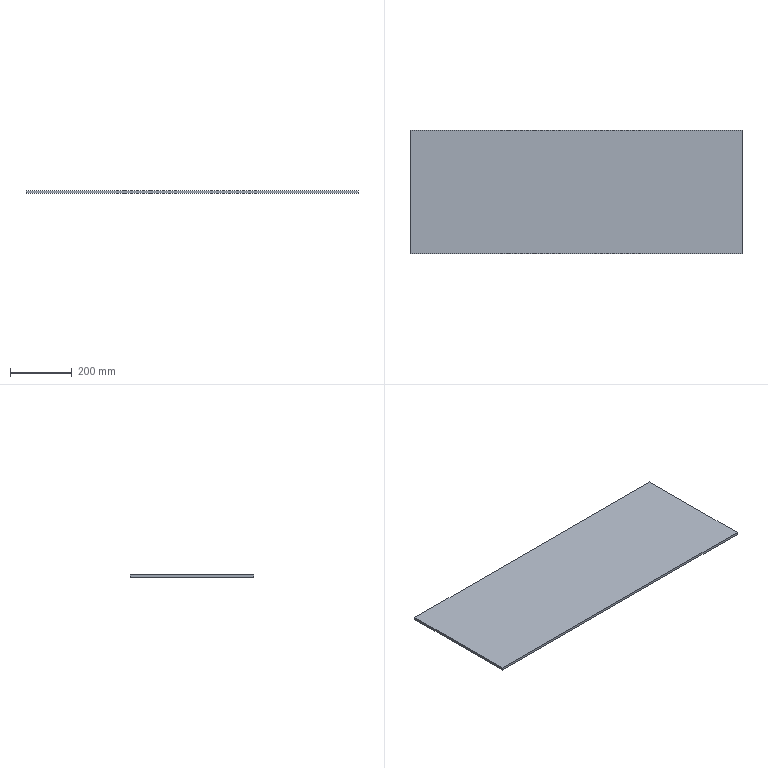Part | STEP file | Rear baffle 1079X402X8_Default<As machined> | 1 solid | 6 faces | box 1079 x 402 x 8 mm | volume 3470064 mm3 | plane 6
STEP:
#1=CARTESIAN_POINT('',(0.,0.,0.));
#2=DIRECTION('',(0.,0.,1.));
#3=DIRECTION('',(1.,0.,0.));
#4=AXIS2_PLACEMENT_3D('',#1,#2,#3);
#5=CARTESIAN_POINT('',(539.5,-201.,0.));
#6=VERTEX_POINT('',#5);
#7=CARTESIAN_POINT('',(539.5,201.,0.));
#8=VERTEX_POINT('',#7);
#9=CARTESIAN_POINT('',(539.5,201.,0.));
#10=DIRECTION('',(0.,1.,0.));
#11=VECTOR('',#10,1.);
#12=LINE('',#9,#11);
#13=CARTESIAN_POINT('',(539.5,201.,8.));
#14=DIRECTION('',(-1.,0.,0.));
#15=DIRECTION('',(0.,0.,1.));
#16=AXIS2_PLACEMENT_3D('',#13,#14,#15);
#17=PLANE('',#16);
#18=CARTESIAN_POINT('',(-8.,0.));
#19=DIRECTION('',(0.,1.));
#20=VECTOR('',#19,1.);
#21=LINE('',#18,#20);
#22=(GEOMETRIC_REPRESENTATION_CONTEXT(2)PARAMETRIC_REPRESENTATION_CONTEXT()REPRESENTATION_CONTEXT('',''));
#23=DEFINITIONAL_REPRESENTATION('',(#21),#22);
#24=PCURVE('',#17,#23);
#25=CARTESIAN_POINT('',(0.,0.,0.));
#26=DIRECTION('',(0.,0.,1.));
#27=DIRECTION('',(1.,0.,0.));
#28=AXIS2_PLACEMENT_3D('',#25,#26,#27);
#29=PLANE('',#28);
#30=CARTESIAN_POINT('',(539.5,201.));
#31=DIRECTION('',(0.,1.));
#32=VECTOR('',#31,1.);
#33=LINE('',#30,#32);
#34=(GEOMETRIC_REPRESENTATION_CONTEXT(2)PARAMETRIC_REPRESENTATION_CONTEXT()REPRESENTATION_CONTEXT('',''));
#35=DEFINITIONAL_REPRESENTATION('',(#33),#34);
#36=PCURVE('',#29,#35);
#37=SURFACE_CURVE('',#12,(#24,#36),.PCURVE_S1.);
#38=EDGE_CURVE('',#6,#8,#37,.T.);
#39=ORIENTED_EDGE('',*,*,#38,.T.);
#40=CARTESIAN_POINT('',(539.5,201.,8.));
#41=VERTEX_POINT('',#40);
#42=CARTESIAN_POINT('',(539.5,201.,8.));
#43=DIRECTION('',(0.,0.,-1.));
#44=VECTOR('',#43,1.);
#45=LINE('',#42,#44);
#46=CARTESIAN_POINT('',(0.,0.));
#47=DIRECTION('',(-1.,0.));
#48=VECTOR('',#47,1.);
#49=LINE('',#46,#48);
#50=(GEOMETRIC_REPRESENTATION_CONTEXT(2)PARAMETRIC_REPRESENTATION_CONTEXT()REPRESENTATION_CONTEXT('',''));
#51=DEFINITIONAL_REPRESENTATION('',(#49),#50);
#52=PCURVE('',#17,#51);
#53=CARTESIAN_POINT('',(-539.5,201.,8.));
#54=DIRECTION('',(0.,-1.,0.));
#55=DIRECTION('',(0.,0.,-1.));
#56=AXIS2_PLACEMENT_3D('',#53,#54,#55);
#57=PLANE('',#56);
#58=CARTESIAN_POINT('',(0.,1079.));
#59=DIRECTION('',(1.,0.));
#60=VECTOR('',#59,1.);
#61=LINE('',#58,#60);
#62=(GEOMETRIC_REPRESENTATION_CONTEXT(2)PARAMETRIC_REPRESENTATION_CONTEXT()REPRESENTATION_CONTEXT('',''));
#63=DEFINITIONAL_REPRESENTATION('',(#61),#62);
#64=PCURVE('',#57,#63);
#65=SURFACE_CURVE('',#45,(#52,#64),.PCURVE_S1.);
#66=EDGE_CURVE('',#41,#8,#65,.T.);
#67=ORIENTED_EDGE('',*,*,#66,.F.);
#68=CARTESIAN_POINT('',(539.5,-201.,8.));
#69=VERTEX_POINT('',#68);
#70=CARTESIAN_POINT('',(539.5,201.,8.));
#71=DIRECTION('',(0.,1.,0.));
#72=VECTOR('',#71,1.);
#73=LINE('',#70,#72);
#74=CARTESIAN_POINT('',(0.,0.));
#75=DIRECTION('',(0.,1.));
#76=VECTOR('',#75,1.);
#77=LINE('',#74,#76);
#78=(GEOMETRIC_REPRESENTATION_CONTEXT(2)PARAMETRIC_REPRESENTATION_CONTEXT()REPRESENTATION_CONTEXT('',''));
#79=DEFINITIONAL_REPRESENTATION('',(#77),#78);
#80=PCURVE('',#17,#79);
#81=CARTESIAN_POINT('',(0.,0.,8.));
#82=DIRECTION('',(0.,0.,1.));
#83=DIRECTION('',(1.,0.,0.));
#84=AXIS2_PLACEMENT_3D('',#81,#82,#83);
#85=PLANE('',#84);
#86=CARTESIAN_POINT('',(539.5,201.));
#87=DIRECTION('',(0.,1.));
#88=VECTOR('',#87,1.);
#89=LINE('',#86,#88);
#90=(GEOMETRIC_REPRESENTATION_CONTEXT(2)PARAMETRIC_REPRESENTATION_CONTEXT()REPRESENTATION_CONTEXT('',''));
#91=DEFINITIONAL_REPRESENTATION('',(#89),#90);
#92=PCURVE('',#85,#91);
#93=SURFACE_CURVE('',#73,(#80,#92),.PCURVE_S1.);
#94=EDGE_CURVE('',#69,#41,#93,.T.);
#95=ORIENTED_EDGE('',*,*,#94,.F.);
#96=CARTESIAN_POINT('',(539.5,-201.,8.));
#97=DIRECTION('',(0.,0.,-1.));
#98=VECTOR('',#97,1.);
#99=LINE('',#96,#98);
#100=CARTESIAN_POINT('',(0.,-402.));
#101=DIRECTION('',(-1.,0.));
#102=VECTOR('',#101,1.);
#103=LINE('',#100,#102);
#104=(GEOMETRIC_REPRESENTATION_CONTEXT(2)PARAMETRIC_REPRESENTATION_CONTEXT()REPRESENTATION_CONTEXT('',''));
#105=DEFINITIONAL_REPRESENTATION('',(#103),#104);
#106=PCURVE('',#17,#105);
#107=CARTESIAN_POINT('',(-539.5,-201.,8.));
#108=DIRECTION('',(0.,1.,0.));
#109=DIRECTION('',(0.,0.,1.));
#110=AXIS2_PLACEMENT_3D('',#107,#108,#109);
#111=PLANE('',#110);
#112=CARTESIAN_POINT('',(0.,1079.));
#113=DIRECTION('',(-1.,0.));
#114=VECTOR('',#113,1.);
#115=LINE('',#112,#114);
#116=(GEOMETRIC_REPRESENTATION_CONTEXT(2)PARAMETRIC_REPRESENTATION_CONTEXT()REPRESENTATION_CONTEXT('',''));
#117=DEFINITIONAL_REPRESENTATION('',(#115),#116);
#118=PCURVE('',#111,#117);
#119=SURFACE_CURVE('',#99,(#106,#118),.PCURVE_S1.);
#120=EDGE_CURVE('',#69,#6,#119,.T.);
#121=ORIENTED_EDGE('',*,*,#120,.T.);
#122=EDGE_LOOP('',(#39,#67,#95,#121));
#123=FACE_BOUND('',#122,.T.);
#124=ADVANCED_FACE('',(#123),#17,.F.);
#125=CARTESIAN_POINT('',(-539.5,201.,0.));
#126=VERTEX_POINT('',#125);
#127=CARTESIAN_POINT('',(-539.5,201.,0.));
#128=DIRECTION('',(-1.,0.,0.));
#129=VECTOR('',#128,1.);
#130=LINE('',#127,#129);
#131=CARTESIAN_POINT('',(8.,0.));
#132=DIRECTION('',(0.,-1.));
#133=VECTOR('',#132,1.);
#134=LINE('',#131,#133);
#135=(GEOMETRIC_REPRESENTATION_CONTEXT(2)PARAMETRIC_REPRESENTATION_CONTEXT()REPRESENTATION_CONTEXT('',''));
#136=DEFINITIONAL_REPRESENTATION('',(#134),#135);
#137=PCURVE('',#57,#136);
#138=CARTESIAN_POINT('',(-539.5,201.));
#139=DIRECTION('',(-1.,0.));
#140=VECTOR('',#139,1.);
#141=LINE('',#138,#140);
#142=(GEOMETRIC_REPRESENTATION_CONTEXT(2)PARAMETRIC_REPRESENTATION_CONTEXT()REPRESENTATION_CONTEXT('',''));
#143=DEFINITIONAL_REPRESENTATION('',(#141),#142);
#144=PCURVE('',#29,#143);
#145=SURFACE_CURVE('',#130,(#137,#144),.PCURVE_S1.);
#146=EDGE_CURVE('',#8,#126,#145,.T.);
#147=ORIENTED_EDGE('',*,*,#146,.T.);
#148=CARTESIAN_POINT('',(-539.5,201.,8.));
#149=VERTEX_POINT('',#148);
#150=CARTESIAN_POINT('',(-539.5,201.,8.));
#151=DIRECTION('',(0.,0.,-1.));
#152=VECTOR('',#151,1.);
#153=LINE('',#150,#152);
#154=CARTESIAN_POINT('',(0.,0.));
#155=DIRECTION('',(1.,0.));
#156=VECTOR('',#155,1.);
#157=LINE('',#154,#156);
#158=(GEOMETRIC_REPRESENTATION_CONTEXT(2)PARAMETRIC_REPRESENTATION_CONTEXT()REPRESENTATION_CONTEXT('',''));
#159=DEFINITIONAL_REPRESENTATION('',(#157),#158);
#160=PCURVE('',#57,#159);
#161=CARTESIAN_POINT('',(-539.5,201.,8.));
#162=DIRECTION('',(1.,0.,0.));
#163=DIRECTION('',(0.,1.,0.));
#164=AXIS2_PLACEMENT_3D('',#161,#162,#163);
#165=PLANE('',#164);
#166=CARTESIAN_POINT('',(0.,0.));
#167=DIRECTION('',(0.,-1.));
#168=VECTOR('',#167,1.);
#169=LINE('',#166,#168);
#170=(GEOMETRIC_REPRESENTATION_CONTEXT(2)PARAMETRIC_REPRESENTATION_CONTEXT()REPRESENTATION_CONTEXT('',''));
#171=DEFINITIONAL_REPRESENTATION('',(#169),#170);
#172=PCURVE('',#165,#171);
#173=SURFACE_CURVE('',#153,(#160,#172),.PCURVE_S1.);
#174=EDGE_CURVE('',#149,#126,#173,.T.);
#175=ORIENTED_EDGE('',*,*,#174,.F.);
#176=CARTESIAN_POINT('',(-539.5,201.,8.));
#177=DIRECTION('',(-1.,0.,0.));
#178=VECTOR('',#177,1.);
#179=LINE('',#176,#178);
#180=CARTESIAN_POINT('',(0.,0.));
#181=DIRECTION('',(0.,-1.));
#182=VECTOR('',#181,1.);
#183=LINE('',#180,#182);
#184=(GEOMETRIC_REPRESENTATION_CONTEXT(2)PARAMETRIC_REPRESENTATION_CONTEXT()REPRESENTATION_CONTEXT('',''));
#185=DEFINITIONAL_REPRESENTATION('',(#183),#184);
#186=PCURVE('',#57,#185);
#187=CARTESIAN_POINT('',(-539.5,201.));
#188=DIRECTION('',(-1.,0.));
#189=VECTOR('',#188,1.);
#190=LINE('',#187,#189);
#191=(GEOMETRIC_REPRESENTATION_CONTEXT(2)PARAMETRIC_REPRESENTATION_CONTEXT()REPRESENTATION_CONTEXT('',''));
#192=DEFINITIONAL_REPRESENTATION('',(#190),#191);
#193=PCURVE('',#85,#192);
#194=SURFACE_CURVE('',#179,(#186,#193),.PCURVE_S1.);
#195=EDGE_CURVE('',#41,#149,#194,.T.);
#196=ORIENTED_EDGE('',*,*,#195,.F.);
#197=ORIENTED_EDGE('',*,*,#66,.T.);
#198=EDGE_LOOP('',(#147,#175,#196,#197));
#199=FACE_BOUND('',#198,.T.);
#200=ADVANCED_FACE('',(#199),#57,.F.);
#201=CARTESIAN_POINT('',(-539.5,-201.,0.));
#202=VERTEX_POINT('',#201);
#203=CARTESIAN_POINT('',(-539.5,201.,0.));
#204=DIRECTION('',(0.,-1.,0.));
#205=VECTOR('',#204,1.);
#206=LINE('',#203,#205);
#207=CARTESIAN_POINT('',(0.,-8.));
#208=DIRECTION('',(-1.,0.));
#209=VECTOR('',#208,1.);
#210=LINE('',#207,#209);
#211=(GEOMETRIC_REPRESENTATION_CONTEXT(2)PARAMETRIC_REPRESENTATION_CONTEXT()REPRESENTATION_CONTEXT('',''));
#212=DEFINITIONAL_REPRESENTATION('',(#210),#211);
#213=PCURVE('',#165,#212);
#214=CARTESIAN_POINT('',(-539.5,201.));
#215=DIRECTION('',(0.,-1.));
#216=VECTOR('',#215,1.);
#217=LINE('',#214,#216);
#218=(GEOMETRIC_REPRESENTATION_CONTEXT(2)PARAMETRIC_REPRESENTATION_CONTEXT()REPRESENTATION_CONTEXT('',''));
#219=DEFINITIONAL_REPRESENTATION('',(#217),#218);
#220=PCURVE('',#29,#219);
#221=SURFACE_CURVE('',#206,(#213,#220),.PCURVE_S1.);
#222=EDGE_CURVE('',#126,#202,#221,.T.);
#223=ORIENTED_EDGE('',*,*,#222,.T.);
#224=CARTESIAN_POINT('',(-539.5,-201.,8.));
#225=VERTEX_POINT('',#224);
#226=CARTESIAN_POINT('',(-539.5,-201.,8.));
#227=DIRECTION('',(0.,0.,-1.));
#228=VECTOR('',#227,1.);
#229=LINE('',#226,#228);
#230=CARTESIAN_POINT('',(-402.,0.));
#231=DIRECTION('',(0.,-1.));
#232=VECTOR('',#231,1.);
#233=LINE('',#230,#232);
#234=(GEOMETRIC_REPRESENTATION_CONTEXT(2)PARAMETRIC_REPRESENTATION_CONTEXT()REPRESENTATION_CONTEXT('',''));
#235=DEFINITIONAL_REPRESENTATION('',(#233),#234);
#236=PCURVE('',#165,#235);
#237=CARTESIAN_POINT('',(0.,0.));
#238=DIRECTION('',(-1.,0.));
#239=VECTOR('',#238,1.);
#240=LINE('',#237,#239);
#241=(GEOMETRIC_REPRESENTATION_CONTEXT(2)PARAMETRIC_REPRESENTATION_CONTEXT()REPRESENTATION_CONTEXT('',''));
#242=DEFINITIONAL_REPRESENTATION('',(#240),#241);
#243=PCURVE('',#111,#242);
#244=SURFACE_CURVE('',#229,(#236,#243),.PCURVE_S1.);
#245=EDGE_CURVE('',#225,#202,#244,.T.);
#246=ORIENTED_EDGE('',*,*,#245,.F.);
#247=CARTESIAN_POINT('',(-539.5,201.,8.));
#248=DIRECTION('',(0.,-1.,0.));
#249=VECTOR('',#248,1.);
#250=LINE('',#247,#249);
#251=CARTESIAN_POINT('',(0.,0.));
#252=DIRECTION('',(-1.,0.));
#253=VECTOR('',#252,1.);
#254=LINE('',#251,#253);
#255=(GEOMETRIC_REPRESENTATION_CONTEXT(2)PARAMETRIC_REPRESENTATION_CONTEXT()REPRESENTATION_CONTEXT('',''));
#256=DEFINITIONAL_REPRESENTATION('',(#254),#255);
#257=PCURVE('',#165,#256);
#258=CARTESIAN_POINT('',(-539.5,201.));
#259=DIRECTION('',(0.,-1.));
#260=VECTOR('',#259,1.);
#261=LINE('',#258,#260);
#262=(GEOMETRIC_REPRESENTATION_CONTEXT(2)PARAMETRIC_REPRESENTATION_CONTEXT()REPRESENTATION_CONTEXT('',''));
#263=DEFINITIONAL_REPRESENTATION('',(#261),#262);
#264=PCURVE('',#85,#263);
#265=SURFACE_CURVE('',#250,(#257,#264),.PCURVE_S1.);
#266=EDGE_CURVE('',#149,#225,#265,.T.);
#267=ORIENTED_EDGE('',*,*,#266,.F.);
#268=ORIENTED_EDGE('',*,*,#174,.T.);
#269=EDGE_LOOP('',(#223,#246,#267,#268));
#270=FACE_BOUND('',#269,.T.);
#271=ADVANCED_FACE('',(#270),#165,.F.);
#272=CARTESIAN_POINT('',(-539.5,-201.,0.));
#273=DIRECTION('',(1.,0.,0.));
#274=VECTOR('',#273,1.);
#275=LINE('',#272,#274);
#276=CARTESIAN_POINT('',(-8.,0.));
#277=DIRECTION('',(0.,1.));
#278=VECTOR('',#277,1.);
#279=LINE('',#276,#278);
#280=(GEOMETRIC_REPRESENTATION_CONTEXT(2)PARAMETRIC_REPRESENTATION_CONTEXT()REPRESENTATION_CONTEXT('',''));
#281=DEFINITIONAL_REPRESENTATION('',(#279),#280);
#282=PCURVE('',#111,#281);
#283=CARTESIAN_POINT('',(-539.5,-201.));
#284=DIRECTION('',(1.,0.));
#285=VECTOR('',#284,1.);
#286=LINE('',#283,#285);
#287=(GEOMETRIC_REPRESENTATION_CONTEXT(2)PARAMETRIC_REPRESENTATION_CONTEXT()REPRESENTATION_CONTEXT('',''));
#288=DEFINITIONAL_REPRESENTATION('',(#286),#287);
#289=PCURVE('',#29,#288);
#290=SURFACE_CURVE('',#275,(#282,#289),.PCURVE_S1.);
#291=EDGE_CURVE('',#202,#6,#290,.T.);
#292=ORIENTED_EDGE('',*,*,#291,.T.);
#293=ORIENTED_EDGE('',*,*,#120,.F.);
#294=CARTESIAN_POINT('',(-539.5,-201.,8.));
#295=DIRECTION('',(1.,0.,0.));
#296=VECTOR('',#295,1.);
#297=LINE('',#294,#296);
#298=CARTESIAN_POINT('',(0.,0.));
#299=DIRECTION('',(0.,1.));
#300=VECTOR('',#299,1.);
#301=LINE('',#298,#300);
#302=(GEOMETRIC_REPRESENTATION_CONTEXT(2)PARAMETRIC_REPRESENTATION_CONTEXT()REPRESENTATION_CONTEXT('',''));
#303=DEFINITIONAL_REPRESENTATION('',(#301),#302);
#304=PCURVE('',#111,#303);
#305=CARTESIAN_POINT('',(-539.5,-201.));
#306=DIRECTION('',(1.,0.));
#307=VECTOR('',#306,1.);
#308=LINE('',#305,#307);
#309=(GEOMETRIC_REPRESENTATION_CONTEXT(2)PARAMETRIC_REPRESENTATION_CONTEXT()REPRESENTATION_CONTEXT('',''));
#310=DEFINITIONAL_REPRESENTATION('',(#308),#309);
#311=PCURVE('',#85,#310);
#312=SURFACE_CURVE('',#297,(#304,#311),.PCURVE_S1.);
#313=EDGE_CURVE('',#225,#69,#312,.T.);
#314=ORIENTED_EDGE('',*,*,#313,.F.);
#315=ORIENTED_EDGE('',*,*,#245,.T.);
#316=EDGE_LOOP('',(#292,#293,#314,#315));
#317=FACE_BOUND('',#316,.T.);
#318=ADVANCED_FACE('',(#317),#111,.F.);
#319=ORIENTED_EDGE('',*,*,#94,.T.);
#320=ORIENTED_EDGE('',*,*,#195,.T.);
#321=ORIENTED_EDGE('',*,*,#266,.T.);
#322=ORIENTED_EDGE('',*,*,#313,.T.);
#323=EDGE_LOOP('',(#319,#320,#321,#322));
#324=FACE_BOUND('',#323,.T.);
#325=ADVANCED_FACE('',(#324),#85,.T.);
#326=ORIENTED_EDGE('',*,*,#38,.F.);
#327=ORIENTED_EDGE('',*,*,#291,.F.);
#328=ORIENTED_EDGE('',*,*,#222,.F.);
#329=ORIENTED_EDGE('',*,*,#146,.F.);
#330=EDGE_LOOP('',(#326,#327,#328,#329));
#331=FACE_BOUND('',#330,.T.);
#332=ADVANCED_FACE('',(#331),#29,.F.);
#333=CLOSED_SHELL('',(#124,#200,#271,#318,#325,#332));
#334=MANIFOLD_SOLID_BREP('',#333);
#335=(LENGTH_UNIT()NAMED_UNIT(*)SI_UNIT(.MILLI.,.METRE.));
#336=UNCERTAINTY_MEASURE_WITH_UNIT(LENGTH_MEASURE(0.0000001),#335,'','');
#337=(NAMED_UNIT(*)PLANE_ANGLE_UNIT()SI_UNIT($,.RADIAN.));
#338=(NAMED_UNIT(*)SI_UNIT($,.STERADIAN.)SOLID_ANGLE_UNIT());
#339=(GEOMETRIC_REPRESENTATION_CONTEXT(3)GLOBAL_UNCERTAINTY_ASSIGNED_CONTEXT((#336))GLOBAL_UNIT_ASSIGNED_CONTEXT((#335,#337,#338))REPRESENTATION_CONTEXT('',''));
#340=ADVANCED_BREP_SHAPE_REPRESENTATION('',(#4,#334),#339);